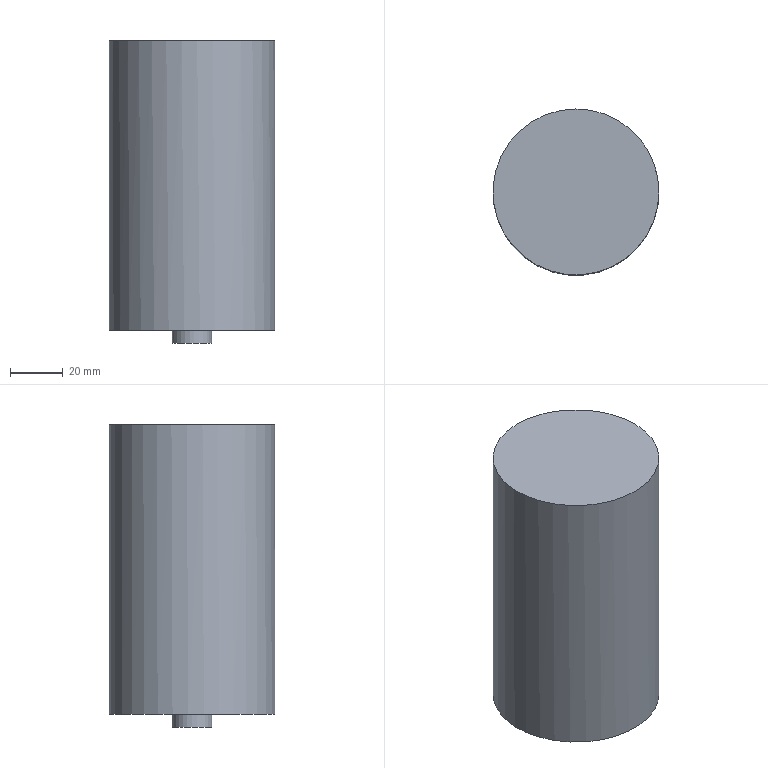Part | NX | features solid 2 | 1 solid | 5 faces | box 63 x 63 x 115 mm | volume 343781 mm3 | plane 3 | cylinder 2 | commonest cylinder face diameters 15 x1 63 x1
STEP:
#1=CARTESIAN_POINT('',(-1147.5,750.,0.));
#2=VERTEX_POINT('',#1);
#3=CARTESIAN_POINT('',(-1140.,750.,0.));
#4=DIRECTION('',(0.,0.,1.));
#5=DIRECTION('',(-1.,0.,0.));
#6=AXIS2_PLACEMENT_3D('',#3,#4,#5);
#7=CIRCLE('',#6,7.5);
#8=EDGE_CURVE('',#2,#2,#7,.T.);
#9=ORIENTED_EDGE('',*,*,#8,.F.);
#10=EDGE_LOOP('',(#9));
#11=FACE_BOUND('',#10,.T.);
#12=CARTESIAN_POINT('',(-1140.,750.,0.));
#13=DIRECTION('',(0.,0.,-1.));
#14=DIRECTION('',(1.,0.,0.));
#15=AXIS2_PLACEMENT_3D('',#12,#13,#14);
#16=PLANE('',#15);
#17=ADVANCED_FACE('',(#11),#16,.T.);
#18=CARTESIAN_POINT('',(-1147.5,750.,5.));
#19=VERTEX_POINT('',#18);
#20=CARTESIAN_POINT('',(-1140.,750.,5.));
#21=DIRECTION('',(0.,0.,1.));
#22=DIRECTION('',(-1.,0.,0.));
#23=AXIS2_PLACEMENT_3D('',#20,#21,#22);
#24=CIRCLE('',#23,7.5);
#25=EDGE_CURVE('',#19,#19,#24,.T.);
#26=ORIENTED_EDGE('',*,*,#25,.F.);
#27=EDGE_LOOP('',(#26));
#28=FACE_BOUND('',#27,.T.);
#29=ORIENTED_EDGE('',*,*,#8,.T.);
#30=EDGE_LOOP('',(#29));
#31=FACE_BOUND('',#30,.T.);
#32=CARTESIAN_POINT('',(-1140.,750.,5.));
#33=DIRECTION('',(0.,0.,1.));
#34=DIRECTION('',(-1.,0.,0.));
#35=AXIS2_PLACEMENT_3D('',#32,#33,#34);
#36=CYLINDRICAL_SURFACE('',#35,7.5);
#37=ADVANCED_FACE('',(#28,#31),#36,.T.);
#38=CARTESIAN_POINT('',(-1108.5,750.,115.));
#39=VERTEX_POINT('',#38);
#40=CARTESIAN_POINT('',(-1140.,750.,115.));
#41=DIRECTION('',(0.,0.,-1.));
#42=DIRECTION('',(1.,0.,0.));
#43=AXIS2_PLACEMENT_3D('',#40,#41,#42);
#44=CIRCLE('',#43,31.5);
#45=EDGE_CURVE('',#39,#39,#44,.T.);
#46=ORIENTED_EDGE('',*,*,#45,.F.);
#47=EDGE_LOOP('',(#46));
#48=FACE_BOUND('',#47,.T.);
#49=CARTESIAN_POINT('',(-1005.,755.,115.));
#50=DIRECTION('',(0.,0.,1.));
#51=DIRECTION('',(1.,0.,0.));
#52=AXIS2_PLACEMENT_3D('',#49,#50,#51);
#53=PLANE('',#52);
#54=ADVANCED_FACE('',(#48),#53,.T.);
#55=ORIENTED_EDGE('',*,*,#25,.T.);
#56=EDGE_LOOP('',(#55));
#57=FACE_BOUND('',#56,.T.);
#58=CARTESIAN_POINT('',(-1140.,781.5,5.));
#59=VERTEX_POINT('',#58);
#60=CARTESIAN_POINT('',(-1140.,750.,5.));
#61=DIRECTION('',(0.,0.,1.));
#62=DIRECTION('',(0.,1.,0.));
#63=AXIS2_PLACEMENT_3D('',#60,#61,#62);
#64=CIRCLE('',#63,31.5);
#65=EDGE_CURVE('',#59,#59,#64,.T.);
#66=ORIENTED_EDGE('',*,*,#65,.F.);
#67=EDGE_LOOP('',(#66));
#68=FACE_BOUND('',#67,.T.);
#69=CARTESIAN_POINT('',(-1140.,750.,5.));
#70=DIRECTION('',(0.,0.,-1.));
#71=DIRECTION('',(1.,0.,0.));
#72=AXIS2_PLACEMENT_3D('',#69,#70,#71);
#73=PLANE('',#72);
#74=ADVANCED_FACE('',(#57,#68),#73,.T.);
#75=ORIENTED_EDGE('',*,*,#45,.T.);
#76=EDGE_LOOP('',(#75));
#77=FACE_BOUND('',#76,.T.);
#78=ORIENTED_EDGE('',*,*,#65,.T.);
#79=EDGE_LOOP('',(#78));
#80=FACE_BOUND('',#79,.T.);
#81=CARTESIAN_POINT('',(-1140.,750.,10.));
#82=DIRECTION('',(0.,0.,1.));
#83=DIRECTION('',(-1.,0.,0.));
#84=AXIS2_PLACEMENT_3D('',#81,#82,#83);
#85=CYLINDRICAL_SURFACE('',#84,31.5);
#86=ADVANCED_FACE('',(#77,#80),#85,.T.);
#87=CLOSED_SHELL('',(#17,#37,#54,#74,#86));
#88=MANIFOLD_SOLID_BREP('',#87);
#89=(LENGTH_UNIT()NAMED_UNIT(*)SI_UNIT(.MILLI.,.METRE.));
#90=UNCERTAINTY_MEASURE_WITH_UNIT(LENGTH_MEASURE(0.00001),#89,'','');
#91=(NAMED_UNIT(*)PLANE_ANGLE_UNIT()SI_UNIT($,.RADIAN.));
#92=(NAMED_UNIT(*)SI_UNIT($,.STERADIAN.)SOLID_ANGLE_UNIT());
#93=(GEOMETRIC_REPRESENTATION_CONTEXT(3)GLOBAL_UNCERTAINTY_ASSIGNED_CONTEXT((#90))GLOBAL_UNIT_ASSIGNED_CONTEXT((#89,#91,#92))REPRESENTATION_CONTEXT('',''));
#94=ADVANCED_BREP_SHAPE_REPRESENTATION('',(#88),#93);